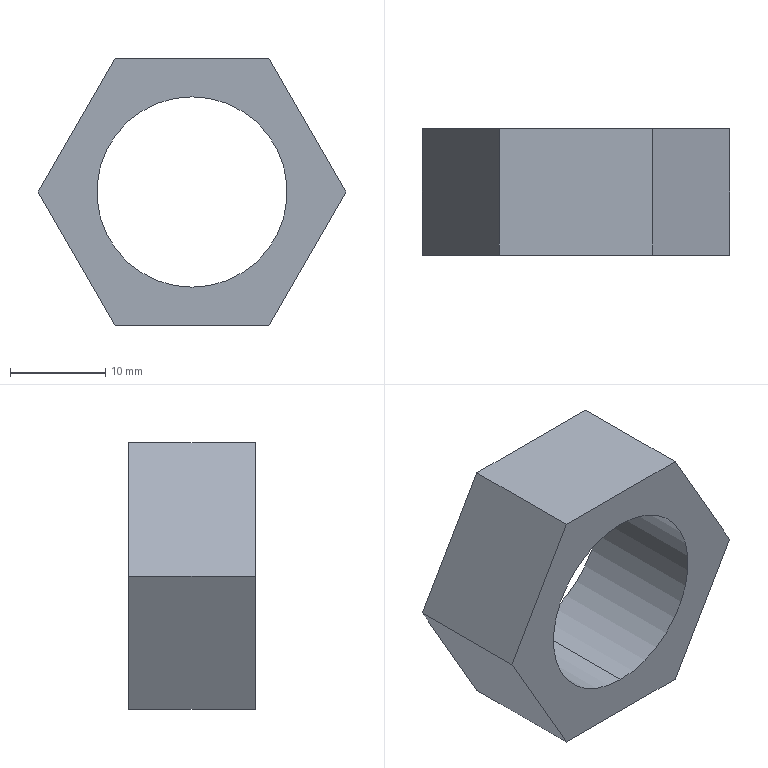Part | STEP file | Pin shaft nut M20 | 1 solid | 10 faces | box 32.332 x 13.3 x 28 mm | volume 4852 mm3 | plane 8 | cylinder 2 | commonest cylinder face diameters 20 x2
STEP:
#1=CARTESIAN_POINT('',(0.,13.3,-10.));
#2=VERTEX_POINT('',#1);
#3=CARTESIAN_POINT('',(0.,13.3,10.));
#4=VERTEX_POINT('',#3);
#5=CARTESIAN_POINT('',(0.,13.3,0.));
#6=DIRECTION('',(0.,1.,0.));
#7=DIRECTION('',(0.,0.,1.));
#8=AXIS2_PLACEMENT_3D('',#5,#6,#7);
#9=CIRCLE('',#8,10.);
#10=EDGE_CURVE('',#2,#4,#9,.T.);
#11=ORIENTED_EDGE('',*,*,#10,.T.);
#12=CARTESIAN_POINT('',(0.,0.,10.));
#13=VERTEX_POINT('',#12);
#14=CARTESIAN_POINT('',(0.,13.3,10.));
#15=DIRECTION('',(0.,-1.,0.));
#16=VECTOR('',#15,1000.);
#17=LINE('',#14,#16);
#18=EDGE_CURVE('',#4,#13,#17,.T.);
#19=ORIENTED_EDGE('',*,*,#18,.T.);
#20=CARTESIAN_POINT('',(0.,0.,-10.));
#21=VERTEX_POINT('',#20);
#22=CARTESIAN_POINT('',(0.,0.,0.));
#23=DIRECTION('',(0.,1.,0.));
#24=DIRECTION('',(0.,0.,1.));
#25=AXIS2_PLACEMENT_3D('',#22,#23,#24);
#26=CIRCLE('',#25,10.);
#27=EDGE_CURVE('',#21,#13,#26,.T.);
#28=ORIENTED_EDGE('',*,*,#27,.F.);
#29=CARTESIAN_POINT('',(0.,13.3,-10.));
#30=DIRECTION('',(0.,-1.,0.));
#31=VECTOR('',#30,1000.);
#32=LINE('',#29,#31);
#33=EDGE_CURVE('',#2,#21,#32,.T.);
#34=ORIENTED_EDGE('',*,*,#33,.F.);
#35=EDGE_LOOP('',(#11,#19,#28,#34));
#36=FACE_OUTER_BOUND('',#35,.T.);
#37=CARTESIAN_POINT('',(0.,13.3,0.));
#38=DIRECTION('',(0.,-1.,0.));
#39=DIRECTION('',(0.,0.,-1.));
#40=AXIS2_PLACEMENT_3D('',#37,#38,#39);
#41=CYLINDRICAL_SURFACE('',#40,10.);
#42=ADVANCED_FACE('',(#36),#41,.F.);
#43=CARTESIAN_POINT('',(-16.166,0.,0.));
#44=VERTEX_POINT('',#43);
#45=CARTESIAN_POINT('',(-8.083,0.,-14.));
#46=VERTEX_POINT('',#45);
#47=CARTESIAN_POINT('',(-12.124,0.,-7.));
#48=DIRECTION('',(0.5,0.,-0.866));
#49=VECTOR('',#48,1000.);
#50=LINE('',#47,#49);
#51=EDGE_CURVE('',#44,#46,#50,.T.);
#52=ORIENTED_EDGE('',*,*,#51,.F.);
#53=CARTESIAN_POINT('',(-16.166,13.3,0.));
#54=VERTEX_POINT('',#53);
#55=CARTESIAN_POINT('',(-16.166,13.3,0.));
#56=DIRECTION('',(0.,-1.,0.));
#57=VECTOR('',#56,1000.);
#58=LINE('',#55,#57);
#59=EDGE_CURVE('',#54,#44,#58,.T.);
#60=ORIENTED_EDGE('',*,*,#59,.F.);
#61=CARTESIAN_POINT('',(-8.083,13.3,-14.));
#62=VERTEX_POINT('',#61);
#63=CARTESIAN_POINT('',(-12.124,13.3,-7.));
#64=DIRECTION('',(0.5,0.,-0.866));
#65=VECTOR('',#64,1000.);
#66=LINE('',#63,#65);
#67=EDGE_CURVE('',#54,#62,#66,.T.);
#68=ORIENTED_EDGE('',*,*,#67,.T.);
#69=CARTESIAN_POINT('',(-8.083,13.3,-14.));
#70=DIRECTION('',(0.,-1.,0.));
#71=VECTOR('',#70,1000.);
#72=LINE('',#69,#71);
#73=EDGE_CURVE('',#62,#46,#72,.T.);
#74=ORIENTED_EDGE('',*,*,#73,.T.);
#75=EDGE_LOOP('',(#52,#60,#68,#74));
#76=FACE_OUTER_BOUND('',#75,.T.);
#77=CARTESIAN_POINT('',(-12.124,13.3,-7.));
#78=DIRECTION('',(-0.866,0.,-0.5));
#79=DIRECTION('',(-0.5,0.,0.866));
#80=AXIS2_PLACEMENT_3D('',#77,#78,#79);
#81=PLANE('',#80);
#82=ADVANCED_FACE('',(#76),#81,.T.);
#83=CARTESIAN_POINT('',(-8.083,0.,14.));
#84=VERTEX_POINT('',#83);
#85=CARTESIAN_POINT('',(-12.124,0.,7.));
#86=DIRECTION('',(-0.5,0.,-0.866));
#87=VECTOR('',#86,1000.);
#88=LINE('',#85,#87);
#89=EDGE_CURVE('',#84,#44,#88,.T.);
#90=ORIENTED_EDGE('',*,*,#89,.F.);
#91=CARTESIAN_POINT('',(-8.083,13.3,14.));
#92=VERTEX_POINT('',#91);
#93=CARTESIAN_POINT('',(-8.083,13.3,14.));
#94=DIRECTION('',(0.,-1.,0.));
#95=VECTOR('',#94,1000.);
#96=LINE('',#93,#95);
#97=EDGE_CURVE('',#92,#84,#96,.T.);
#98=ORIENTED_EDGE('',*,*,#97,.F.);
#99=CARTESIAN_POINT('',(-12.124,13.3,7.));
#100=DIRECTION('',(-0.5,0.,-0.866));
#101=VECTOR('',#100,1000.);
#102=LINE('',#99,#101);
#103=EDGE_CURVE('',#92,#54,#102,.T.);
#104=ORIENTED_EDGE('',*,*,#103,.T.);
#105=ORIENTED_EDGE('',*,*,#59,.T.);
#106=EDGE_LOOP('',(#90,#98,#104,#105));
#107=FACE_OUTER_BOUND('',#106,.T.);
#108=CARTESIAN_POINT('',(-12.124,13.3,7.));
#109=DIRECTION('',(-0.866,0.,0.5));
#110=DIRECTION('',(0.5,0.,0.866));
#111=AXIS2_PLACEMENT_3D('',#108,#109,#110);
#112=PLANE('',#111);
#113=ADVANCED_FACE('',(#107),#112,.T.);
#114=CARTESIAN_POINT('',(8.083,0.,14.));
#115=VERTEX_POINT('',#114);
#116=CARTESIAN_POINT('',(0.,0.,14.));
#117=DIRECTION('',(-1.,0.,0.));
#118=VECTOR('',#117,1000.);
#119=LINE('',#116,#118);
#120=EDGE_CURVE('',#115,#84,#119,.T.);
#121=ORIENTED_EDGE('',*,*,#120,.F.);
#122=CARTESIAN_POINT('',(8.083,13.3,14.));
#123=VERTEX_POINT('',#122);
#124=CARTESIAN_POINT('',(8.083,13.3,14.));
#125=DIRECTION('',(0.,-1.,0.));
#126=VECTOR('',#125,1000.);
#127=LINE('',#124,#126);
#128=EDGE_CURVE('',#123,#115,#127,.T.);
#129=ORIENTED_EDGE('',*,*,#128,.F.);
#130=CARTESIAN_POINT('',(0.,13.3,14.));
#131=DIRECTION('',(-1.,0.,0.));
#132=VECTOR('',#131,1000.);
#133=LINE('',#130,#132);
#134=EDGE_CURVE('',#123,#92,#133,.T.);
#135=ORIENTED_EDGE('',*,*,#134,.T.);
#136=ORIENTED_EDGE('',*,*,#97,.T.);
#137=EDGE_LOOP('',(#121,#129,#135,#136));
#138=FACE_OUTER_BOUND('',#137,.T.);
#139=CARTESIAN_POINT('',(0.,13.3,14.));
#140=DIRECTION('',(0.,0.,1.));
#141=DIRECTION('',(1.,0.,0.));
#142=AXIS2_PLACEMENT_3D('',#139,#140,#141);
#143=PLANE('',#142);
#144=ADVANCED_FACE('',(#138),#143,.T.);
#145=CARTESIAN_POINT('',(16.166,0.,0.));
#146=VERTEX_POINT('',#145);
#147=CARTESIAN_POINT('',(12.124,0.,7.));
#148=DIRECTION('',(-0.5,0.,0.866));
#149=VECTOR('',#148,1000.);
#150=LINE('',#147,#149);
#151=EDGE_CURVE('',#146,#115,#150,.T.);
#152=ORIENTED_EDGE('',*,*,#151,.F.);
#153=CARTESIAN_POINT('',(16.166,13.3,0.));
#154=VERTEX_POINT('',#153);
#155=CARTESIAN_POINT('',(16.166,13.3,0.));
#156=DIRECTION('',(0.,-1.,0.));
#157=VECTOR('',#156,1000.);
#158=LINE('',#155,#157);
#159=EDGE_CURVE('',#154,#146,#158,.T.);
#160=ORIENTED_EDGE('',*,*,#159,.F.);
#161=CARTESIAN_POINT('',(12.124,13.3,7.));
#162=DIRECTION('',(-0.5,0.,0.866));
#163=VECTOR('',#162,1000.);
#164=LINE('',#161,#163);
#165=EDGE_CURVE('',#154,#123,#164,.T.);
#166=ORIENTED_EDGE('',*,*,#165,.T.);
#167=ORIENTED_EDGE('',*,*,#128,.T.);
#168=EDGE_LOOP('',(#152,#160,#166,#167));
#169=FACE_OUTER_BOUND('',#168,.T.);
#170=CARTESIAN_POINT('',(12.124,13.3,7.));
#171=DIRECTION('',(0.866,0.,0.5));
#172=DIRECTION('',(0.5,0.,-0.866));
#173=AXIS2_PLACEMENT_3D('',#170,#171,#172);
#174=PLANE('',#173);
#175=ADVANCED_FACE('',(#169),#174,.T.);
#176=CARTESIAN_POINT('',(8.083,0.,-14.));
#177=VERTEX_POINT('',#176);
#178=CARTESIAN_POINT('',(12.124,0.,-7.));
#179=DIRECTION('',(0.5,0.,0.866));
#180=VECTOR('',#179,1000.);
#181=LINE('',#178,#180);
#182=EDGE_CURVE('',#177,#146,#181,.T.);
#183=ORIENTED_EDGE('',*,*,#182,.F.);
#184=CARTESIAN_POINT('',(8.083,13.3,-14.));
#185=VERTEX_POINT('',#184);
#186=CARTESIAN_POINT('',(8.083,13.3,-14.));
#187=DIRECTION('',(0.,-1.,0.));
#188=VECTOR('',#187,1000.);
#189=LINE('',#186,#188);
#190=EDGE_CURVE('',#185,#177,#189,.T.);
#191=ORIENTED_EDGE('',*,*,#190,.F.);
#192=CARTESIAN_POINT('',(12.124,13.3,-7.));
#193=DIRECTION('',(0.5,0.,0.866));
#194=VECTOR('',#193,1000.);
#195=LINE('',#192,#194);
#196=EDGE_CURVE('',#185,#154,#195,.T.);
#197=ORIENTED_EDGE('',*,*,#196,.T.);
#198=ORIENTED_EDGE('',*,*,#159,.T.);
#199=EDGE_LOOP('',(#183,#191,#197,#198));
#200=FACE_OUTER_BOUND('',#199,.T.);
#201=CARTESIAN_POINT('',(12.124,13.3,-7.));
#202=DIRECTION('',(0.866,0.,-0.5));
#203=DIRECTION('',(-0.5,0.,-0.866));
#204=AXIS2_PLACEMENT_3D('',#201,#202,#203);
#205=PLANE('',#204);
#206=ADVANCED_FACE('',(#200),#205,.T.);
#207=CARTESIAN_POINT('',(0.,0.,-14.));
#208=DIRECTION('',(1.,0.,0.));
#209=VECTOR('',#208,1000.);
#210=LINE('',#207,#209);
#211=EDGE_CURVE('',#46,#177,#210,.T.);
#212=ORIENTED_EDGE('',*,*,#211,.F.);
#213=ORIENTED_EDGE('',*,*,#73,.F.);
#214=CARTESIAN_POINT('',(0.,13.3,-14.));
#215=DIRECTION('',(1.,0.,0.));
#216=VECTOR('',#215,1000.);
#217=LINE('',#214,#216);
#218=EDGE_CURVE('',#62,#185,#217,.T.);
#219=ORIENTED_EDGE('',*,*,#218,.T.);
#220=ORIENTED_EDGE('',*,*,#190,.T.);
#221=EDGE_LOOP('',(#212,#213,#219,#220));
#222=FACE_OUTER_BOUND('',#221,.T.);
#223=CARTESIAN_POINT('',(0.,13.3,-14.));
#224=DIRECTION('',(0.,0.,-1.));
#225=DIRECTION('',(-1.,0.,0.));
#226=AXIS2_PLACEMENT_3D('',#223,#224,#225);
#227=PLANE('',#226);
#228=ADVANCED_FACE('',(#222),#227,.T.);
#229=ORIENTED_EDGE('',*,*,#10,.F.);
#230=CARTESIAN_POINT('',(0.,13.3,0.));
#231=DIRECTION('',(0.,1.,0.));
#232=DIRECTION('',(0.,0.,1.));
#233=AXIS2_PLACEMENT_3D('',#230,#231,#232);
#234=CIRCLE('',#233,10.);
#235=EDGE_CURVE('',#4,#2,#234,.T.);
#236=ORIENTED_EDGE('',*,*,#235,.F.);
#237=EDGE_LOOP('',(#229,#236));
#238=FACE_BOUND('',#237,.T.);
#239=ORIENTED_EDGE('',*,*,#67,.F.);
#240=ORIENTED_EDGE('',*,*,#103,.F.);
#241=ORIENTED_EDGE('',*,*,#134,.F.);
#242=ORIENTED_EDGE('',*,*,#165,.F.);
#243=ORIENTED_EDGE('',*,*,#196,.F.);
#244=ORIENTED_EDGE('',*,*,#218,.F.);
#245=EDGE_LOOP('',(#239,#240,#241,#242,#243,#244));
#246=FACE_OUTER_BOUND('',#245,.T.);
#247=CARTESIAN_POINT('',(0.,13.3,0.));
#248=DIRECTION('',(0.,1.,0.));
#249=DIRECTION('',(0.,0.,1.));
#250=AXIS2_PLACEMENT_3D('',#247,#248,#249);
#251=PLANE('',#250);
#252=ADVANCED_FACE('',(#238,#246),#251,.T.);
#253=ORIENTED_EDGE('',*,*,#27,.T.);
#254=CARTESIAN_POINT('',(0.,0.,0.));
#255=DIRECTION('',(0.,1.,0.));
#256=DIRECTION('',(0.,0.,1.));
#257=AXIS2_PLACEMENT_3D('',#254,#255,#256);
#258=CIRCLE('',#257,10.);
#259=EDGE_CURVE('',#13,#21,#258,.T.);
#260=ORIENTED_EDGE('',*,*,#259,.T.);
#261=EDGE_LOOP('',(#253,#260));
#262=FACE_BOUND('',#261,.T.);
#263=ORIENTED_EDGE('',*,*,#51,.T.);
#264=ORIENTED_EDGE('',*,*,#211,.T.);
#265=ORIENTED_EDGE('',*,*,#182,.T.);
#266=ORIENTED_EDGE('',*,*,#151,.T.);
#267=ORIENTED_EDGE('',*,*,#120,.T.);
#268=ORIENTED_EDGE('',*,*,#89,.T.);
#269=EDGE_LOOP('',(#263,#264,#265,#266,#267,#268));
#270=FACE_OUTER_BOUND('',#269,.T.);
#271=CARTESIAN_POINT('',(0.,0.,0.));
#272=DIRECTION('',(0.,1.,0.));
#273=DIRECTION('',(0.,0.,1.));
#274=AXIS2_PLACEMENT_3D('',#271,#272,#273);
#275=PLANE('',#274);
#276=ADVANCED_FACE('',(#262,#270),#275,.F.);
#277=ORIENTED_EDGE('',*,*,#18,.F.);
#278=ORIENTED_EDGE('',*,*,#235,.T.);
#279=ORIENTED_EDGE('',*,*,#33,.T.);
#280=ORIENTED_EDGE('',*,*,#259,.F.);
#281=EDGE_LOOP('',(#277,#278,#279,#280));
#282=FACE_OUTER_BOUND('',#281,.T.);
#283=CARTESIAN_POINT('',(0.,13.3,0.));
#284=DIRECTION('',(0.,-1.,0.));
#285=DIRECTION('',(0.,0.,-1.));
#286=AXIS2_PLACEMENT_3D('',#283,#284,#285);
#287=CYLINDRICAL_SURFACE('',#286,10.);
#288=ADVANCED_FACE('',(#282),#287,.F.);
#289=CLOSED_SHELL('',(#42,#82,#113,#144,#175,#206,#228,#252,#276,#288));
#290=MANIFOLD_SOLID_BREP('',#289);
#291=CARTESIAN_POINT('',(0.,0.,0.));
#292=DIRECTION('',(0.,0.,1.));
#293=DIRECTION('',(1.,0.,0.));
#294=AXIS2_PLACEMENT_3D('',#291,#292,#293);
#295=(LENGTH_UNIT()NAMED_UNIT(*)SI_UNIT(.MILLI.,.METRE.));
#296=UNCERTAINTY_MEASURE_WITH_UNIT(LENGTH_MEASURE(0.00001),#295,'','');
#297=(NAMED_UNIT(*)PLANE_ANGLE_UNIT()SI_UNIT($,.RADIAN.));
#298=(NAMED_UNIT(*)SI_UNIT($,.STERADIAN.)SOLID_ANGLE_UNIT());
#299=(GEOMETRIC_REPRESENTATION_CONTEXT(3)GLOBAL_UNCERTAINTY_ASSIGNED_CONTEXT((#296))GLOBAL_UNIT_ASSIGNED_CONTEXT((#295,#297,#298))REPRESENTATION_CONTEXT('',''));
#300=ADVANCED_BREP_SHAPE_REPRESENTATION('',(#290,#294),#299);